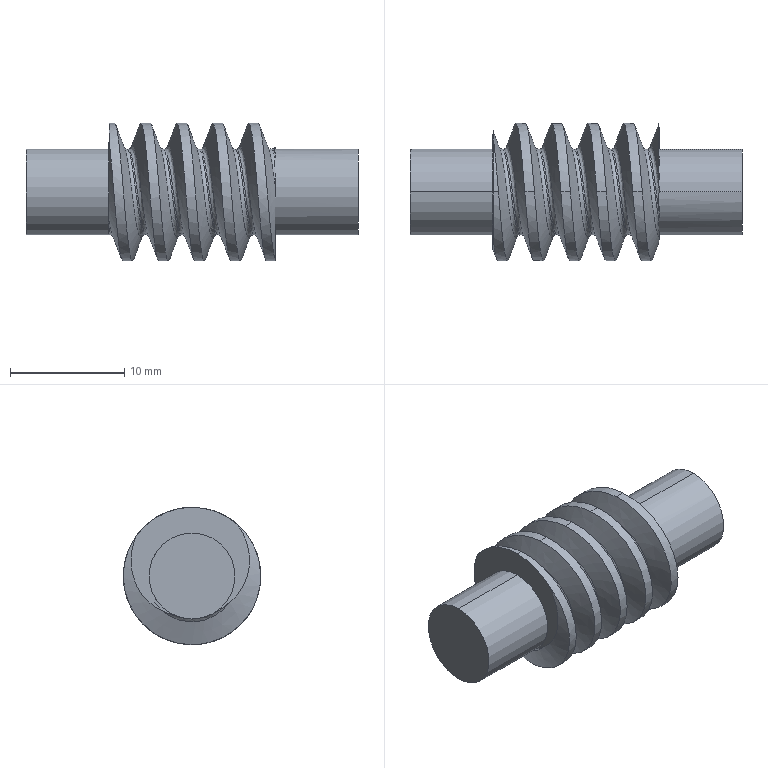Part | SolidWorks | features BaseBody 1 | 1 solid | 24 faces | box 29 x 12 x 12 mm | volume 1793 mm3 | cylinder 15 | spline 5 | plane 4 | commonest cylinder face diameters 12 x11 7.5 x4